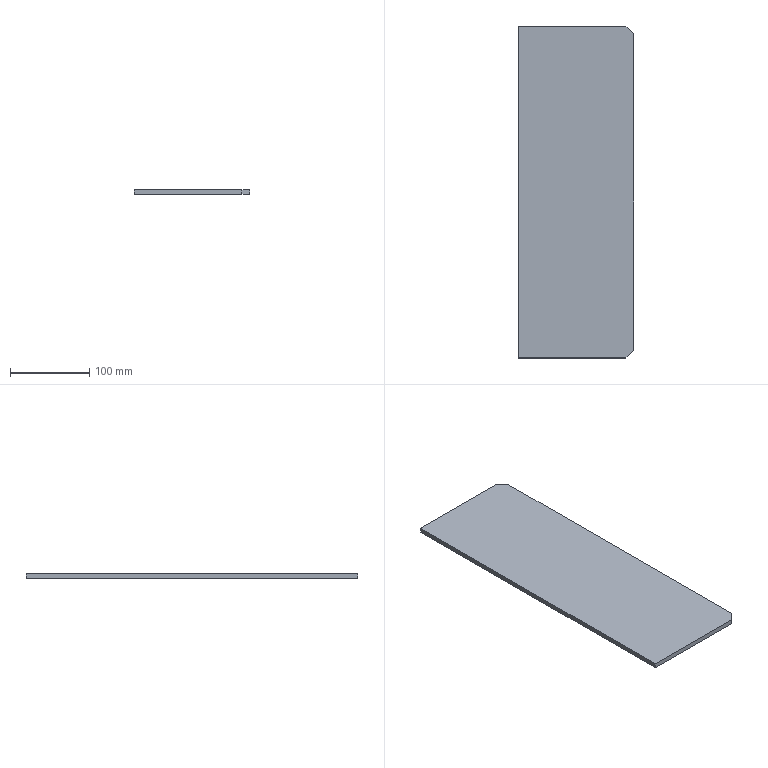Part | STEP file | 03-Rib plate 1 | 1 solid | 8 faces | box 146 x 419 x 6 mm | volume 366444 mm3 | plane 8
STEP:
#1=CARTESIAN_POINT('',(0.,0.,0.));
#2=DIRECTION('',(0.,0.,1.));
#3=DIRECTION('',(1.,0.,0.));
#4=AXIS2_PLACEMENT_3D('',#1,#2,#3);
#5=CARTESIAN_POINT('',(0.,0.,0.));
#6=VERTEX_POINT('',#5);
#7=CARTESIAN_POINT('',(0.,-419.,0.));
#8=VERTEX_POINT('',#7);
#9=CARTESIAN_POINT('',(0.,0.,0.));
#10=DIRECTION('',(0.,-1.,0.));
#11=VECTOR('',#10,1.);
#12=LINE('',#9,#11);
#13=CARTESIAN_POINT('',(0.,0.,6.));
#14=DIRECTION('',(1.,0.,0.));
#15=DIRECTION('',(0.,1.,0.));
#16=AXIS2_PLACEMENT_3D('',#13,#14,#15);
#17=PLANE('',#16);
#18=CARTESIAN_POINT('',(0.,-6.));
#19=DIRECTION('',(-1.,0.));
#20=VECTOR('',#19,1.);
#21=LINE('',#18,#20);
#22=(GEOMETRIC_REPRESENTATION_CONTEXT(2)PARAMETRIC_REPRESENTATION_CONTEXT()REPRESENTATION_CONTEXT('',''));
#23=DEFINITIONAL_REPRESENTATION('',(#21),#22);
#24=PCURVE('',#17,#23);
#25=CARTESIAN_POINT('',(0.,0.,0.));
#26=DIRECTION('',(0.,0.,1.));
#27=DIRECTION('',(1.,0.,0.));
#28=AXIS2_PLACEMENT_3D('',#25,#26,#27);
#29=PLANE('',#28);
#30=CARTESIAN_POINT('',(0.,0.));
#31=DIRECTION('',(0.,-1.));
#32=VECTOR('',#31,1.);
#33=LINE('',#30,#32);
#34=(GEOMETRIC_REPRESENTATION_CONTEXT(2)PARAMETRIC_REPRESENTATION_CONTEXT()REPRESENTATION_CONTEXT('',''));
#35=DEFINITIONAL_REPRESENTATION('',(#33),#34);
#36=PCURVE('',#29,#35);
#37=SURFACE_CURVE('',#12,(#24,#36),.PCURVE_S1.);
#38=EDGE_CURVE('',#6,#8,#37,.T.);
#39=ORIENTED_EDGE('',*,*,#38,.T.);
#40=CARTESIAN_POINT('',(0.,-419.,6.));
#41=VERTEX_POINT('',#40);
#42=CARTESIAN_POINT('',(0.,-419.,6.));
#43=DIRECTION('',(0.,0.,-1.));
#44=VECTOR('',#43,1.);
#45=LINE('',#42,#44);
#46=CARTESIAN_POINT('',(-419.,0.));
#47=DIRECTION('',(0.,-1.));
#48=VECTOR('',#47,1.);
#49=LINE('',#46,#48);
#50=(GEOMETRIC_REPRESENTATION_CONTEXT(2)PARAMETRIC_REPRESENTATION_CONTEXT()REPRESENTATION_CONTEXT('',''));
#51=DEFINITIONAL_REPRESENTATION('',(#49),#50);
#52=PCURVE('',#17,#51);
#53=CARTESIAN_POINT('',(0.,-419.,6.));
#54=DIRECTION('',(0.,1.,0.));
#55=DIRECTION('',(0.,0.,1.));
#56=AXIS2_PLACEMENT_3D('',#53,#54,#55);
#57=PLANE('',#56);
#58=CARTESIAN_POINT('',(0.,0.));
#59=DIRECTION('',(-1.,0.));
#60=VECTOR('',#59,1.);
#61=LINE('',#58,#60);
#62=(GEOMETRIC_REPRESENTATION_CONTEXT(2)PARAMETRIC_REPRESENTATION_CONTEXT()REPRESENTATION_CONTEXT('',''));
#63=DEFINITIONAL_REPRESENTATION('',(#61),#62);
#64=PCURVE('',#57,#63);
#65=SURFACE_CURVE('',#45,(#52,#64),.PCURVE_S1.);
#66=EDGE_CURVE('',#41,#8,#65,.T.);
#67=ORIENTED_EDGE('',*,*,#66,.F.);
#68=CARTESIAN_POINT('',(0.,0.,6.));
#69=VERTEX_POINT('',#68);
#70=CARTESIAN_POINT('',(0.,0.,6.));
#71=DIRECTION('',(0.,-1.,0.));
#72=VECTOR('',#71,1.);
#73=LINE('',#70,#72);
#74=CARTESIAN_POINT('',(0.,0.));
#75=DIRECTION('',(-1.,0.));
#76=VECTOR('',#75,1.);
#77=LINE('',#74,#76);
#78=(GEOMETRIC_REPRESENTATION_CONTEXT(2)PARAMETRIC_REPRESENTATION_CONTEXT()REPRESENTATION_CONTEXT('',''));
#79=DEFINITIONAL_REPRESENTATION('',(#77),#78);
#80=PCURVE('',#17,#79);
#81=CARTESIAN_POINT('',(0.,0.,6.));
#82=DIRECTION('',(0.,0.,1.));
#83=DIRECTION('',(1.,0.,0.));
#84=AXIS2_PLACEMENT_3D('',#81,#82,#83);
#85=PLANE('',#84);
#86=CARTESIAN_POINT('',(0.,0.));
#87=DIRECTION('',(0.,-1.));
#88=VECTOR('',#87,1.);
#89=LINE('',#86,#88);
#90=(GEOMETRIC_REPRESENTATION_CONTEXT(2)PARAMETRIC_REPRESENTATION_CONTEXT()REPRESENTATION_CONTEXT('',''));
#91=DEFINITIONAL_REPRESENTATION('',(#89),#90);
#92=PCURVE('',#85,#91);
#93=SURFACE_CURVE('',#73,(#80,#92),.PCURVE_S1.);
#94=EDGE_CURVE('',#69,#41,#93,.T.);
#95=ORIENTED_EDGE('',*,*,#94,.F.);
#96=CARTESIAN_POINT('',(0.,0.,6.));
#97=DIRECTION('',(0.,0.,-1.));
#98=VECTOR('',#97,1.);
#99=LINE('',#96,#98);
#100=CARTESIAN_POINT('',(0.,0.));
#101=DIRECTION('',(0.,-1.));
#102=VECTOR('',#101,1.);
#103=LINE('',#100,#102);
#104=(GEOMETRIC_REPRESENTATION_CONTEXT(2)PARAMETRIC_REPRESENTATION_CONTEXT()REPRESENTATION_CONTEXT('',''));
#105=DEFINITIONAL_REPRESENTATION('',(#103),#104);
#106=PCURVE('',#17,#105);
#107=CARTESIAN_POINT('',(0.,0.,6.));
#108=DIRECTION('',(0.,-1.,0.));
#109=DIRECTION('',(0.,0.,-1.));
#110=AXIS2_PLACEMENT_3D('',#107,#108,#109);
#111=PLANE('',#110);
#112=CARTESIAN_POINT('',(0.,0.));
#113=DIRECTION('',(1.,0.));
#114=VECTOR('',#113,1.);
#115=LINE('',#112,#114);
#116=(GEOMETRIC_REPRESENTATION_CONTEXT(2)PARAMETRIC_REPRESENTATION_CONTEXT()REPRESENTATION_CONTEXT('',''));
#117=DEFINITIONAL_REPRESENTATION('',(#115),#116);
#118=PCURVE('',#111,#117);
#119=SURFACE_CURVE('',#99,(#106,#118),.PCURVE_S1.);
#120=EDGE_CURVE('',#69,#6,#119,.T.);
#121=ORIENTED_EDGE('',*,*,#120,.T.);
#122=EDGE_LOOP('',(#39,#67,#95,#121));
#123=FACE_BOUND('',#122,.T.);
#124=ADVANCED_FACE('',(#123),#17,.F.);
#125=CARTESIAN_POINT('',(136.,-419.,0.));
#126=VERTEX_POINT('',#125);
#127=CARTESIAN_POINT('',(0.,-419.,0.));
#128=DIRECTION('',(1.,0.,0.));
#129=VECTOR('',#128,1.);
#130=LINE('',#127,#129);
#131=CARTESIAN_POINT('',(-6.,0.));
#132=DIRECTION('',(0.,1.));
#133=VECTOR('',#132,1.);
#134=LINE('',#131,#133);
#135=(GEOMETRIC_REPRESENTATION_CONTEXT(2)PARAMETRIC_REPRESENTATION_CONTEXT()REPRESENTATION_CONTEXT('',''));
#136=DEFINITIONAL_REPRESENTATION('',(#134),#135);
#137=PCURVE('',#57,#136);
#138=CARTESIAN_POINT('',(0.,-419.));
#139=DIRECTION('',(1.,0.));
#140=VECTOR('',#139,1.);
#141=LINE('',#138,#140);
#142=(GEOMETRIC_REPRESENTATION_CONTEXT(2)PARAMETRIC_REPRESENTATION_CONTEXT()REPRESENTATION_CONTEXT('',''));
#143=DEFINITIONAL_REPRESENTATION('',(#141),#142);
#144=PCURVE('',#29,#143);
#145=SURFACE_CURVE('',#130,(#137,#144),.PCURVE_S1.);
#146=EDGE_CURVE('',#8,#126,#145,.T.);
#147=ORIENTED_EDGE('',*,*,#146,.T.);
#148=CARTESIAN_POINT('',(136.,-419.,6.));
#149=VERTEX_POINT('',#148);
#150=CARTESIAN_POINT('',(136.,-419.,6.));
#151=DIRECTION('',(0.,0.,-1.));
#152=VECTOR('',#151,1.);
#153=LINE('',#150,#152);
#154=CARTESIAN_POINT('',(0.,136.));
#155=DIRECTION('',(-1.,0.));
#156=VECTOR('',#155,1.);
#157=LINE('',#154,#156);
#158=(GEOMETRIC_REPRESENTATION_CONTEXT(2)PARAMETRIC_REPRESENTATION_CONTEXT()REPRESENTATION_CONTEXT('',''));
#159=DEFINITIONAL_REPRESENTATION('',(#157),#158);
#160=PCURVE('',#57,#159);
#161=CARTESIAN_POINT('',(146.,-409.,6.));
#162=DIRECTION('',(-0.7071,0.7071,0.));
#163=DIRECTION('',(-0.7071,-0.7071,0.));
#164=AXIS2_PLACEMENT_3D('',#161,#162,#163);
#165=PLANE('',#164);
#166=CARTESIAN_POINT('',(14.142,0.));
#167=DIRECTION('',(0.,-1.));
#168=VECTOR('',#167,1.);
#169=LINE('',#166,#168);
#170=(GEOMETRIC_REPRESENTATION_CONTEXT(2)PARAMETRIC_REPRESENTATION_CONTEXT()REPRESENTATION_CONTEXT('',''));
#171=DEFINITIONAL_REPRESENTATION('',(#169),#170);
#172=PCURVE('',#165,#171);
#173=SURFACE_CURVE('',#153,(#160,#172),.PCURVE_S1.);
#174=EDGE_CURVE('',#149,#126,#173,.T.);
#175=ORIENTED_EDGE('',*,*,#174,.F.);
#176=CARTESIAN_POINT('',(0.,-419.,6.));
#177=DIRECTION('',(1.,0.,0.));
#178=VECTOR('',#177,1.);
#179=LINE('',#176,#178);
#180=CARTESIAN_POINT('',(0.,0.));
#181=DIRECTION('',(0.,1.));
#182=VECTOR('',#181,1.);
#183=LINE('',#180,#182);
#184=(GEOMETRIC_REPRESENTATION_CONTEXT(2)PARAMETRIC_REPRESENTATION_CONTEXT()REPRESENTATION_CONTEXT('',''));
#185=DEFINITIONAL_REPRESENTATION('',(#183),#184);
#186=PCURVE('',#57,#185);
#187=CARTESIAN_POINT('',(0.,-419.));
#188=DIRECTION('',(1.,0.));
#189=VECTOR('',#188,1.);
#190=LINE('',#187,#189);
#191=(GEOMETRIC_REPRESENTATION_CONTEXT(2)PARAMETRIC_REPRESENTATION_CONTEXT()REPRESENTATION_CONTEXT('',''));
#192=DEFINITIONAL_REPRESENTATION('',(#190),#191);
#193=PCURVE('',#85,#192);
#194=SURFACE_CURVE('',#179,(#186,#193),.PCURVE_S1.);
#195=EDGE_CURVE('',#41,#149,#194,.T.);
#196=ORIENTED_EDGE('',*,*,#195,.F.);
#197=ORIENTED_EDGE('',*,*,#66,.T.);
#198=EDGE_LOOP('',(#147,#175,#196,#197));
#199=FACE_BOUND('',#198,.T.);
#200=ADVANCED_FACE('',(#199),#57,.F.);
#201=CARTESIAN_POINT('',(146.,-409.,0.));
#202=VERTEX_POINT('',#201);
#203=CARTESIAN_POINT('',(146.,-409.,0.));
#204=DIRECTION('',(0.7071,0.7071,0.));
#205=VECTOR('',#204,1.);
#206=LINE('',#203,#205);
#207=CARTESIAN_POINT('',(0.,-6.));
#208=DIRECTION('',(-1.,0.));
#209=VECTOR('',#208,1.);
#210=LINE('',#207,#209);
#211=(GEOMETRIC_REPRESENTATION_CONTEXT(2)PARAMETRIC_REPRESENTATION_CONTEXT()REPRESENTATION_CONTEXT('',''));
#212=DEFINITIONAL_REPRESENTATION('',(#210),#211);
#213=PCURVE('',#165,#212);
#214=CARTESIAN_POINT('',(146.,-409.));
#215=DIRECTION('',(0.7071,0.7071));
#216=VECTOR('',#215,1.);
#217=LINE('',#214,#216);
#218=(GEOMETRIC_REPRESENTATION_CONTEXT(2)PARAMETRIC_REPRESENTATION_CONTEXT()REPRESENTATION_CONTEXT('',''));
#219=DEFINITIONAL_REPRESENTATION('',(#217),#218);
#220=PCURVE('',#29,#219);
#221=SURFACE_CURVE('',#206,(#213,#220),.PCURVE_S1.);
#222=EDGE_CURVE('',#126,#202,#221,.T.);
#223=ORIENTED_EDGE('',*,*,#222,.T.);
#224=CARTESIAN_POINT('',(146.,-409.,6.));
#225=VERTEX_POINT('',#224);
#226=CARTESIAN_POINT('',(146.,-409.,6.));
#227=DIRECTION('',(0.,0.,-1.));
#228=VECTOR('',#227,1.);
#229=LINE('',#226,#228);
#230=CARTESIAN_POINT('',(0.,0.));
#231=DIRECTION('',(0.,-1.));
#232=VECTOR('',#231,1.);
#233=LINE('',#230,#232);
#234=(GEOMETRIC_REPRESENTATION_CONTEXT(2)PARAMETRIC_REPRESENTATION_CONTEXT()REPRESENTATION_CONTEXT('',''));
#235=DEFINITIONAL_REPRESENTATION('',(#233),#234);
#236=PCURVE('',#165,#235);
#237=CARTESIAN_POINT('',(146.,-10.,6.));
#238=DIRECTION('',(-1.,0.,0.));
#239=DIRECTION('',(0.,-1.,0.));
#240=AXIS2_PLACEMENT_3D('',#237,#238,#239);
#241=PLANE('',#240);
#242=CARTESIAN_POINT('',(399.,0.));
#243=DIRECTION('',(0.,-1.));
#244=VECTOR('',#243,1.);
#245=LINE('',#242,#244);
#246=(GEOMETRIC_REPRESENTATION_CONTEXT(2)PARAMETRIC_REPRESENTATION_CONTEXT()REPRESENTATION_CONTEXT('',''));
#247=DEFINITIONAL_REPRESENTATION('',(#245),#246);
#248=PCURVE('',#241,#247);
#249=SURFACE_CURVE('',#229,(#236,#248),.PCURVE_S1.);
#250=EDGE_CURVE('',#225,#202,#249,.T.);
#251=ORIENTED_EDGE('',*,*,#250,.F.);
#252=CARTESIAN_POINT('',(146.,-409.,6.));
#253=DIRECTION('',(0.7071,0.7071,0.));
#254=VECTOR('',#253,1.);
#255=LINE('',#252,#254);
#256=CARTESIAN_POINT('',(0.,0.));
#257=DIRECTION('',(-1.,0.));
#258=VECTOR('',#257,1.);
#259=LINE('',#256,#258);
#260=(GEOMETRIC_REPRESENTATION_CONTEXT(2)PARAMETRIC_REPRESENTATION_CONTEXT()REPRESENTATION_CONTEXT('',''));
#261=DEFINITIONAL_REPRESENTATION('',(#259),#260);
#262=PCURVE('',#165,#261);
#263=CARTESIAN_POINT('',(146.,-409.));
#264=DIRECTION('',(0.7071,0.7071));
#265=VECTOR('',#264,1.);
#266=LINE('',#263,#265);
#267=(GEOMETRIC_REPRESENTATION_CONTEXT(2)PARAMETRIC_REPRESENTATION_CONTEXT()REPRESENTATION_CONTEXT('',''));
#268=DEFINITIONAL_REPRESENTATION('',(#266),#267);
#269=PCURVE('',#85,#268);
#270=SURFACE_CURVE('',#255,(#262,#269),.PCURVE_S1.);
#271=EDGE_CURVE('',#149,#225,#270,.T.);
#272=ORIENTED_EDGE('',*,*,#271,.F.);
#273=ORIENTED_EDGE('',*,*,#174,.T.);
#274=EDGE_LOOP('',(#223,#251,#272,#273));
#275=FACE_BOUND('',#274,.T.);
#276=ADVANCED_FACE('',(#275),#165,.F.);
#277=CARTESIAN_POINT('',(146.,-10.,0.));
#278=VERTEX_POINT('',#277);
#279=CARTESIAN_POINT('',(146.,-10.,0.));
#280=DIRECTION('',(0.,1.,0.));
#281=VECTOR('',#280,1.);
#282=LINE('',#279,#281);
#283=CARTESIAN_POINT('',(0.,-6.));
#284=DIRECTION('',(-1.,0.));
#285=VECTOR('',#284,1.);
#286=LINE('',#283,#285);
#287=(GEOMETRIC_REPRESENTATION_CONTEXT(2)PARAMETRIC_REPRESENTATION_CONTEXT()REPRESENTATION_CONTEXT('',''));
#288=DEFINITIONAL_REPRESENTATION('',(#286),#287);
#289=PCURVE('',#241,#288);
#290=CARTESIAN_POINT('',(146.,-10.));
#291=DIRECTION('',(0.,1.));
#292=VECTOR('',#291,1.);
#293=LINE('',#290,#292);
#294=(GEOMETRIC_REPRESENTATION_CONTEXT(2)PARAMETRIC_REPRESENTATION_CONTEXT()REPRESENTATION_CONTEXT('',''));
#295=DEFINITIONAL_REPRESENTATION('',(#293),#294);
#296=PCURVE('',#29,#295);
#297=SURFACE_CURVE('',#282,(#289,#296),.PCURVE_S1.);
#298=EDGE_CURVE('',#202,#278,#297,.T.);
#299=ORIENTED_EDGE('',*,*,#298,.T.);
#300=CARTESIAN_POINT('',(146.,-10.,6.));
#301=VERTEX_POINT('',#300);
#302=CARTESIAN_POINT('',(146.,-10.,6.));
#303=DIRECTION('',(0.,0.,-1.));
#304=VECTOR('',#303,1.);
#305=LINE('',#302,#304);
#306=CARTESIAN_POINT('',(0.,0.));
#307=DIRECTION('',(0.,-1.));
#308=VECTOR('',#307,1.);
#309=LINE('',#306,#308);
#310=(GEOMETRIC_REPRESENTATION_CONTEXT(2)PARAMETRIC_REPRESENTATION_CONTEXT()REPRESENTATION_CONTEXT('',''));
#311=DEFINITIONAL_REPRESENTATION('',(#309),#310);
#312=PCURVE('',#241,#311);
#313=CARTESIAN_POINT('',(136.,0.,6.));
#314=DIRECTION('',(-0.7071,-0.7071,0.));
#315=DIRECTION('',(0.7071,-0.7071,0.));
#316=AXIS2_PLACEMENT_3D('',#313,#314,#315);
#317=PLANE('',#316);
#318=CARTESIAN_POINT('',(14.142,0.));
#319=DIRECTION('',(0.,-1.));
#320=VECTOR('',#319,1.);
#321=LINE('',#318,#320);
#322=(GEOMETRIC_REPRESENTATION_CONTEXT(2)PARAMETRIC_REPRESENTATION_CONTEXT()REPRESENTATION_CONTEXT('',''));
#323=DEFINITIONAL_REPRESENTATION('',(#321),#322);
#324=PCURVE('',#317,#323);
#325=SURFACE_CURVE('',#305,(#312,#324),.PCURVE_S1.);
#326=EDGE_CURVE('',#301,#278,#325,.T.);
#327=ORIENTED_EDGE('',*,*,#326,.F.);
#328=CARTESIAN_POINT('',(146.,-10.,6.));
#329=DIRECTION('',(0.,1.,0.));
#330=VECTOR('',#329,1.);
#331=LINE('',#328,#330);
#332=CARTESIAN_POINT('',(0.,0.));
#333=DIRECTION('',(-1.,0.));
#334=VECTOR('',#333,1.);
#335=LINE('',#332,#334);
#336=(GEOMETRIC_REPRESENTATION_CONTEXT(2)PARAMETRIC_REPRESENTATION_CONTEXT()REPRESENTATION_CONTEXT('',''));
#337=DEFINITIONAL_REPRESENTATION('',(#335),#336);
#338=PCURVE('',#241,#337);
#339=CARTESIAN_POINT('',(146.,-10.));
#340=DIRECTION('',(0.,1.));
#341=VECTOR('',#340,1.);
#342=LINE('',#339,#341);
#343=(GEOMETRIC_REPRESENTATION_CONTEXT(2)PARAMETRIC_REPRESENTATION_CONTEXT()REPRESENTATION_CONTEXT('',''));
#344=DEFINITIONAL_REPRESENTATION('',(#342),#343);
#345=PCURVE('',#85,#344);
#346=SURFACE_CURVE('',#331,(#338,#345),.PCURVE_S1.);
#347=EDGE_CURVE('',#225,#301,#346,.T.);
#348=ORIENTED_EDGE('',*,*,#347,.F.);
#349=ORIENTED_EDGE('',*,*,#250,.T.);
#350=EDGE_LOOP('',(#299,#327,#348,#349));
#351=FACE_BOUND('',#350,.T.);
#352=ADVANCED_FACE('',(#351),#241,.F.);
#353=CARTESIAN_POINT('',(136.,0.,0.));
#354=VERTEX_POINT('',#353);
#355=CARTESIAN_POINT('',(136.,0.,0.));
#356=DIRECTION('',(-0.7071,0.7071,0.));
#357=VECTOR('',#356,1.);
#358=LINE('',#355,#357);
#359=CARTESIAN_POINT('',(0.,-6.));
#360=DIRECTION('',(-1.,0.));
#361=VECTOR('',#360,1.);
#362=LINE('',#359,#361);
#363=(GEOMETRIC_REPRESENTATION_CONTEXT(2)PARAMETRIC_REPRESENTATION_CONTEXT()REPRESENTATION_CONTEXT('',''));
#364=DEFINITIONAL_REPRESENTATION('',(#362),#363);
#365=PCURVE('',#317,#364);
#366=CARTESIAN_POINT('',(136.,0.));
#367=DIRECTION('',(-0.7071,0.7071));
#368=VECTOR('',#367,1.);
#369=LINE('',#366,#368);
#370=(GEOMETRIC_REPRESENTATION_CONTEXT(2)PARAMETRIC_REPRESENTATION_CONTEXT()REPRESENTATION_CONTEXT('',''));
#371=DEFINITIONAL_REPRESENTATION('',(#369),#370);
#372=PCURVE('',#29,#371);
#373=SURFACE_CURVE('',#358,(#365,#372),.PCURVE_S1.);
#374=EDGE_CURVE('',#278,#354,#373,.T.);
#375=ORIENTED_EDGE('',*,*,#374,.T.);
#376=CARTESIAN_POINT('',(136.,0.,6.));
#377=VERTEX_POINT('',#376);
#378=CARTESIAN_POINT('',(136.,0.,6.));
#379=DIRECTION('',(0.,0.,-1.));
#380=VECTOR('',#379,1.);
#381=LINE('',#378,#380);
#382=CARTESIAN_POINT('',(0.,0.));
#383=DIRECTION('',(0.,-1.));
#384=VECTOR('',#383,1.);
#385=LINE('',#382,#384);
#386=(GEOMETRIC_REPRESENTATION_CONTEXT(2)PARAMETRIC_REPRESENTATION_CONTEXT()REPRESENTATION_CONTEXT('',''));
#387=DEFINITIONAL_REPRESENTATION('',(#385),#386);
#388=PCURVE('',#317,#387);
#389=CARTESIAN_POINT('',(0.,136.));
#390=DIRECTION('',(1.,0.));
#391=VECTOR('',#390,1.);
#392=LINE('',#389,#391);
#393=(GEOMETRIC_REPRESENTATION_CONTEXT(2)PARAMETRIC_REPRESENTATION_CONTEXT()REPRESENTATION_CONTEXT('',''));
#394=DEFINITIONAL_REPRESENTATION('',(#392),#393);
#395=PCURVE('',#111,#394);
#396=SURFACE_CURVE('',#381,(#388,#395),.PCURVE_S1.);
#397=EDGE_CURVE('',#377,#354,#396,.T.);
#398=ORIENTED_EDGE('',*,*,#397,.F.);
#399=CARTESIAN_POINT('',(136.,0.,6.));
#400=DIRECTION('',(-0.7071,0.7071,0.));
#401=VECTOR('',#400,1.);
#402=LINE('',#399,#401);
#403=CARTESIAN_POINT('',(0.,0.));
#404=DIRECTION('',(-1.,0.));
#405=VECTOR('',#404,1.);
#406=LINE('',#403,#405);
#407=(GEOMETRIC_REPRESENTATION_CONTEXT(2)PARAMETRIC_REPRESENTATION_CONTEXT()REPRESENTATION_CONTEXT('',''));
#408=DEFINITIONAL_REPRESENTATION('',(#406),#407);
#409=PCURVE('',#317,#408);
#410=CARTESIAN_POINT('',(136.,0.));
#411=DIRECTION('',(-0.7071,0.7071));
#412=VECTOR('',#411,1.);
#413=LINE('',#410,#412);
#414=(GEOMETRIC_REPRESENTATION_CONTEXT(2)PARAMETRIC_REPRESENTATION_CONTEXT()REPRESENTATION_CONTEXT('',''));
#415=DEFINITIONAL_REPRESENTATION('',(#413),#414);
#416=PCURVE('',#85,#415);
#417=SURFACE_CURVE('',#402,(#409,#416),.PCURVE_S1.);
#418=EDGE_CURVE('',#301,#377,#417,.T.);
#419=ORIENTED_EDGE('',*,*,#418,.F.);
#420=ORIENTED_EDGE('',*,*,#326,.T.);
#421=EDGE_LOOP('',(#375,#398,#419,#420));
#422=FACE_BOUND('',#421,.T.);
#423=ADVANCED_FACE('',(#422),#317,.F.);
#424=CARTESIAN_POINT('',(0.,0.,0.));
#425=DIRECTION('',(-1.,0.,0.));
#426=VECTOR('',#425,1.);
#427=LINE('',#424,#426);
#428=CARTESIAN_POINT('',(6.,0.));
#429=DIRECTION('',(0.,-1.));
#430=VECTOR('',#429,1.);
#431=LINE('',#428,#430);
#432=(GEOMETRIC_REPRESENTATION_CONTEXT(2)PARAMETRIC_REPRESENTATION_CONTEXT()REPRESENTATION_CONTEXT('',''));
#433=DEFINITIONAL_REPRESENTATION('',(#431),#432);
#434=PCURVE('',#111,#433);
#435=CARTESIAN_POINT('',(0.,0.));
#436=DIRECTION('',(-1.,0.));
#437=VECTOR('',#436,1.);
#438=LINE('',#435,#437);
#439=(GEOMETRIC_REPRESENTATION_CONTEXT(2)PARAMETRIC_REPRESENTATION_CONTEXT()REPRESENTATION_CONTEXT('',''));
#440=DEFINITIONAL_REPRESENTATION('',(#438),#439);
#441=PCURVE('',#29,#440);
#442=SURFACE_CURVE('',#427,(#434,#441),.PCURVE_S1.);
#443=EDGE_CURVE('',#354,#6,#442,.T.);
#444=ORIENTED_EDGE('',*,*,#443,.T.);
#445=ORIENTED_EDGE('',*,*,#120,.F.);
#446=CARTESIAN_POINT('',(0.,0.,6.));
#447=DIRECTION('',(-1.,0.,0.));
#448=VECTOR('',#447,1.);
#449=LINE('',#446,#448);
#450=CARTESIAN_POINT('',(0.,0.));
#451=DIRECTION('',(0.,-1.));
#452=VECTOR('',#451,1.);
#453=LINE('',#450,#452);
#454=(GEOMETRIC_REPRESENTATION_CONTEXT(2)PARAMETRIC_REPRESENTATION_CONTEXT()REPRESENTATION_CONTEXT('',''));
#455=DEFINITIONAL_REPRESENTATION('',(#453),#454);
#456=PCURVE('',#111,#455);
#457=CARTESIAN_POINT('',(0.,0.));
#458=DIRECTION('',(-1.,0.));
#459=VECTOR('',#458,1.);
#460=LINE('',#457,#459);
#461=(GEOMETRIC_REPRESENTATION_CONTEXT(2)PARAMETRIC_REPRESENTATION_CONTEXT()REPRESENTATION_CONTEXT('',''));
#462=DEFINITIONAL_REPRESENTATION('',(#460),#461);
#463=PCURVE('',#85,#462);
#464=SURFACE_CURVE('',#449,(#456,#463),.PCURVE_S1.);
#465=EDGE_CURVE('',#377,#69,#464,.T.);
#466=ORIENTED_EDGE('',*,*,#465,.F.);
#467=ORIENTED_EDGE('',*,*,#397,.T.);
#468=EDGE_LOOP('',(#444,#445,#466,#467));
#469=FACE_BOUND('',#468,.T.);
#470=ADVANCED_FACE('',(#469),#111,.F.);
#471=ORIENTED_EDGE('',*,*,#94,.T.);
#472=ORIENTED_EDGE('',*,*,#195,.T.);
#473=ORIENTED_EDGE('',*,*,#271,.T.);
#474=ORIENTED_EDGE('',*,*,#347,.T.);
#475=ORIENTED_EDGE('',*,*,#418,.T.);
#476=ORIENTED_EDGE('',*,*,#465,.T.);
#477=EDGE_LOOP('',(#471,#472,#473,#474,#475,#476));
#478=FACE_BOUND('',#477,.T.);
#479=ADVANCED_FACE('',(#478),#85,.T.);
#480=ORIENTED_EDGE('',*,*,#38,.F.);
#481=ORIENTED_EDGE('',*,*,#443,.F.);
#482=ORIENTED_EDGE('',*,*,#374,.F.);
#483=ORIENTED_EDGE('',*,*,#298,.F.);
#484=ORIENTED_EDGE('',*,*,#222,.F.);
#485=ORIENTED_EDGE('',*,*,#146,.F.);
#486=EDGE_LOOP('',(#480,#481,#482,#483,#484,#485));
#487=FACE_BOUND('',#486,.T.);
#488=ADVANCED_FACE('',(#487),#29,.F.);
#489=CLOSED_SHELL('',(#124,#200,#276,#352,#423,#470,#479,#488));
#490=MANIFOLD_SOLID_BREP('',#489);
#491=(LENGTH_UNIT()NAMED_UNIT(*)SI_UNIT(.MILLI.,.METRE.));
#492=UNCERTAINTY_MEASURE_WITH_UNIT(LENGTH_MEASURE(0.0000001),#491,'','');
#493=(NAMED_UNIT(*)PLANE_ANGLE_UNIT()SI_UNIT($,.RADIAN.));
#494=(NAMED_UNIT(*)SI_UNIT($,.STERADIAN.)SOLID_ANGLE_UNIT());
#495=(GEOMETRIC_REPRESENTATION_CONTEXT(3)GLOBAL_UNCERTAINTY_ASSIGNED_CONTEXT((#492))GLOBAL_UNIT_ASSIGNED_CONTEXT((#491,#493,#494))REPRESENTATION_CONTEXT('',''));
#496=ADVANCED_BREP_SHAPE_REPRESENTATION('',(#4,#490),#495);